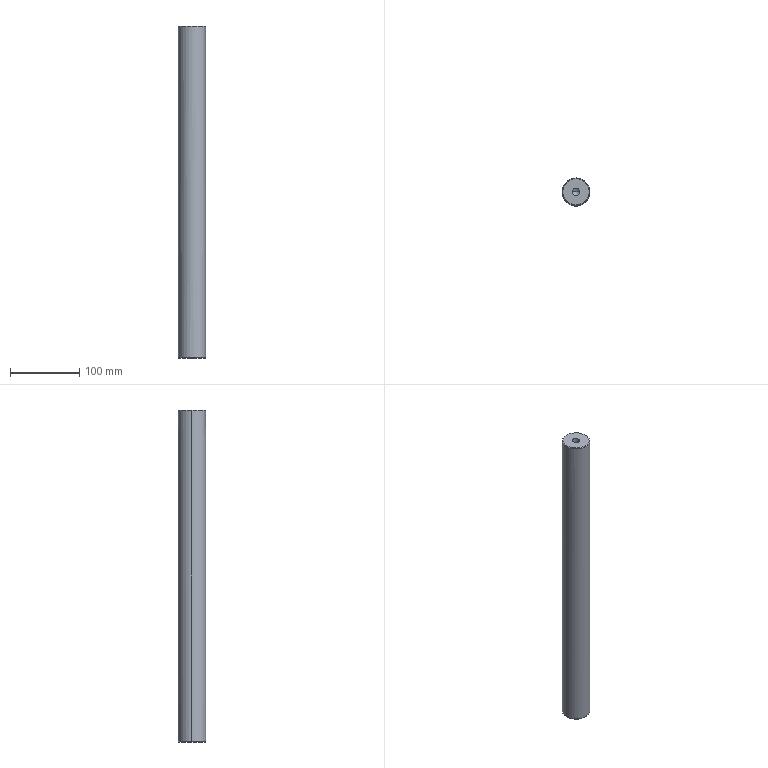Part | SolidWorks | features BaseBody 1 | 1 solid | 12 faces | box 40 x 40 x 480 mm | volume 600589 mm3 | cone 6 | cylinder 4 | plane 2 | commonest cylinder face diameters 10.2 x2 40 x2
STEP:
#1=CARTESIAN_POINT('',(0.,20.,479.));
#2=VERTEX_POINT('',#1);
#3=CARTESIAN_POINT('',(20.,0.,479.));
#4=VERTEX_POINT('',#3);
#5=CARTESIAN_POINT('',(0.,0.,479.));
#6=DIRECTION('',(0.,0.,-1.));
#7=DIRECTION('',(-1.,0.,0.));
#8=AXIS2_PLACEMENT_3D('',#5,#6,#7);
#9=CIRCLE('',#8,20.);
#10=EDGE_CURVE('',#2,#4,#9,.T.);
#11=ORIENTED_EDGE('',*,*,#10,.T.);
#12=CARTESIAN_POINT('',(20.,0.,1.));
#13=VERTEX_POINT('',#12);
#14=CARTESIAN_POINT('',(20.,0.,480.));
#15=DIRECTION('',(0.,0.,-1.));
#16=VECTOR('',#15,1000.);
#17=LINE('',#14,#16);
#18=EDGE_CURVE('',#4,#13,#17,.T.);
#19=ORIENTED_EDGE('',*,*,#18,.T.);
#20=CARTESIAN_POINT('',(-20.,0.,1.));
#21=VERTEX_POINT('',#20);
#22=CARTESIAN_POINT('',(0.,0.,1.));
#23=DIRECTION('',(0.,0.,1.));
#24=DIRECTION('',(-1.,0.,0.));
#25=AXIS2_PLACEMENT_3D('',#22,#23,#24);
#26=CIRCLE('',#25,20.);
#27=EDGE_CURVE('',#13,#21,#26,.T.);
#28=ORIENTED_EDGE('',*,*,#27,.T.);
#29=CARTESIAN_POINT('',(-20.,0.,479.));
#30=VERTEX_POINT('',#29);
#31=CARTESIAN_POINT('',(-20.,0.,480.));
#32=DIRECTION('',(0.,0.,-1.));
#33=VECTOR('',#32,1000.);
#34=LINE('',#31,#33);
#35=EDGE_CURVE('',#30,#21,#34,.T.);
#36=ORIENTED_EDGE('',*,*,#35,.F.);
#37=CARTESIAN_POINT('',(0.,0.,479.));
#38=DIRECTION('',(0.,0.,-1.));
#39=DIRECTION('',(-1.,0.,0.));
#40=AXIS2_PLACEMENT_3D('',#37,#38,#39);
#41=CIRCLE('',#40,20.);
#42=EDGE_CURVE('',#30,#2,#41,.T.);
#43=ORIENTED_EDGE('',*,*,#42,.T.);
#44=EDGE_LOOP('',(#11,#19,#28,#36,#43));
#45=FACE_OUTER_BOUND('',#44,.T.);
#46=CARTESIAN_POINT('',(0.,0.,480.));
#47=DIRECTION('',(0.,0.,-1.));
#48=DIRECTION('',(-1.,0.,0.));
#49=AXIS2_PLACEMENT_3D('',#46,#47,#48);
#50=CYLINDRICAL_SURFACE('',#49,20.);
#51=ADVANCED_FACE('',(#45),#50,.T.);
#52=CARTESIAN_POINT('',(19.,0.,0.));
#53=VERTEX_POINT('',#52);
#54=CARTESIAN_POINT('',(-19.,0.,0.));
#55=VERTEX_POINT('',#54);
#56=CARTESIAN_POINT('',(0.,0.,0.));
#57=DIRECTION('',(0.,0.,1.));
#58=DIRECTION('',(1.,0.,0.));
#59=AXIS2_PLACEMENT_3D('',#56,#57,#58);
#60=CIRCLE('',#59,19.);
#61=EDGE_CURVE('',#53,#55,#60,.T.);
#62=ORIENTED_EDGE('',*,*,#61,.T.);
#63=CARTESIAN_POINT('',(-20.,0.,1.));
#64=DIRECTION('',(-0.7071,0.,0.7071));
#65=VECTOR('',#64,1000.);
#66=LINE('',#63,#65);
#67=EDGE_CURVE('',#55,#21,#66,.T.);
#68=ORIENTED_EDGE('',*,*,#67,.T.);
#69=ORIENTED_EDGE('',*,*,#27,.F.);
#70=CARTESIAN_POINT('',(20.,0.,1.));
#71=DIRECTION('',(0.7071,0.,0.7071));
#72=VECTOR('',#71,1000.);
#73=LINE('',#70,#72);
#74=EDGE_CURVE('',#53,#13,#73,.T.);
#75=ORIENTED_EDGE('',*,*,#74,.F.);
#76=EDGE_LOOP('',(#62,#68,#69,#75));
#77=FACE_OUTER_BOUND('',#76,.T.);
#78=CARTESIAN_POINT('',(0.,0.,1.));
#79=DIRECTION('',(0.,0.,1.));
#80=DIRECTION('',(1.,0.,0.));
#81=AXIS2_PLACEMENT_3D('',#78,#79,#80);
#82=CONICAL_SURFACE('',#81,20.,0.7854);
#83=ADVANCED_FACE('',(#77),#82,.T.);
#84=CARTESIAN_POINT('',(0.,19.,480.));
#85=VERTEX_POINT('',#84);
#86=CARTESIAN_POINT('',(0.,-19.,480.));
#87=VERTEX_POINT('',#86);
#88=CARTESIAN_POINT('',(0.,0.,480.));
#89=DIRECTION('',(0.,0.,-1.));
#90=DIRECTION('',(0.,1.,0.));
#91=AXIS2_PLACEMENT_3D('',#88,#89,#90);
#92=CIRCLE('',#91,19.);
#93=EDGE_CURVE('',#85,#87,#92,.T.);
#94=ORIENTED_EDGE('',*,*,#93,.T.);
#95=CARTESIAN_POINT('',(0.,-20.,479.));
#96=VERTEX_POINT('',#95);
#97=CARTESIAN_POINT('',(0.,-20.,479.));
#98=DIRECTION('',(0.,-0.7071,-0.7071));
#99=VECTOR('',#98,1000.);
#100=LINE('',#97,#99);
#101=EDGE_CURVE('',#87,#96,#100,.T.);
#102=ORIENTED_EDGE('',*,*,#101,.T.);
#103=CARTESIAN_POINT('',(0.,0.,479.));
#104=DIRECTION('',(0.,0.,-1.));
#105=DIRECTION('',(-1.,0.,0.));
#106=AXIS2_PLACEMENT_3D('',#103,#104,#105);
#107=CIRCLE('',#106,20.);
#108=EDGE_CURVE('',#4,#96,#107,.T.);
#109=ORIENTED_EDGE('',*,*,#108,.F.);
#110=ORIENTED_EDGE('',*,*,#10,.F.);
#111=CARTESIAN_POINT('',(0.,20.,479.));
#112=DIRECTION('',(0.,0.7071,-0.7071));
#113=VECTOR('',#112,1000.);
#114=LINE('',#111,#113);
#115=EDGE_CURVE('',#85,#2,#114,.T.);
#116=ORIENTED_EDGE('',*,*,#115,.F.);
#117=EDGE_LOOP('',(#94,#102,#109,#110,#116));
#118=FACE_OUTER_BOUND('',#117,.T.);
#119=CARTESIAN_POINT('',(0.,0.,479.));
#120=DIRECTION('',(0.,0.,-1.));
#121=DIRECTION('',(0.,1.,0.));
#122=AXIS2_PLACEMENT_3D('',#119,#120,#121);
#123=CONICAL_SURFACE('',#122,20.,0.7854);
#124=ADVANCED_FACE('',(#118),#123,.T.);
#125=CARTESIAN_POINT('',(-5.1,0.,450.75));
#126=VERTEX_POINT('',#125);
#127=CARTESIAN_POINT('',(5.1,0.,450.75));
#128=VERTEX_POINT('',#127);
#129=CARTESIAN_POINT('',(0.,0.,450.75));
#130=DIRECTION('',(0.,0.,1.));
#131=DIRECTION('',(1.,0.,0.));
#132=AXIS2_PLACEMENT_3D('',#129,#130,#131);
#133=CIRCLE('',#132,5.1);
#134=EDGE_CURVE('',#126,#128,#133,.T.);
#135=ORIENTED_EDGE('',*,*,#134,.F.);
#136=CARTESIAN_POINT('',(-5.1,0.,480.));
#137=VERTEX_POINT('',#136);
#138=CARTESIAN_POINT('',(-5.1,0.,480.));
#139=DIRECTION('',(0.,0.,1.));
#140=VECTOR('',#139,1000.);
#141=LINE('',#138,#140);
#142=EDGE_CURVE('',#126,#137,#141,.T.);
#143=ORIENTED_EDGE('',*,*,#142,.T.);
#144=CARTESIAN_POINT('',(5.1,0.,480.));
#145=VERTEX_POINT('',#144);
#146=CARTESIAN_POINT('',(0.,0.,480.));
#147=DIRECTION('',(0.,0.,-1.));
#148=DIRECTION('',(1.,0.,0.));
#149=AXIS2_PLACEMENT_3D('',#146,#147,#148);
#150=CIRCLE('',#149,5.1);
#151=EDGE_CURVE('',#145,#137,#150,.T.);
#152=ORIENTED_EDGE('',*,*,#151,.F.);
#153=CARTESIAN_POINT('',(5.1,0.,480.));
#154=DIRECTION('',(0.,0.,1.));
#155=VECTOR('',#154,1000.);
#156=LINE('',#153,#155);
#157=EDGE_CURVE('',#128,#145,#156,.T.);
#158=ORIENTED_EDGE('',*,*,#157,.F.);
#159=EDGE_LOOP('',(#135,#143,#152,#158));
#160=FACE_OUTER_BOUND('',#159,.T.);
#161=CARTESIAN_POINT('',(0.,0.,480.));
#162=DIRECTION('',(0.,0.,1.));
#163=DIRECTION('',(1.,0.,0.));
#164=AXIS2_PLACEMENT_3D('',#161,#162,#163);
#165=CYLINDRICAL_SURFACE('',#164,5.1);
#166=ADVANCED_FACE('',(#160),#165,.F.);
#167=CARTESIAN_POINT('',(0.,0.,447.686));
#168=VERTEX_POINT('',#167);
#169=CARTESIAN_POINT('',(5.1,0.,450.75));
#170=DIRECTION('',(0.8572,0.,0.515));
#171=VECTOR('',#170,1000.);
#172=LINE('',#169,#171);
#173=EDGE_CURVE('',#168,#128,#172,.T.);
#174=ORIENTED_EDGE('',*,*,#173,.F.);
#175=CARTESIAN_POINT('',(-5.1,0.,450.75));
#176=DIRECTION('',(-0.8572,0.,0.515));
#177=VECTOR('',#176,1000.);
#178=LINE('',#175,#177);
#179=EDGE_CURVE('',#168,#126,#178,.T.);
#180=ORIENTED_EDGE('',*,*,#179,.T.);
#181=ORIENTED_EDGE('',*,*,#134,.T.);
#182=EDGE_LOOP('',(#174,#180,#181));
#183=FACE_OUTER_BOUND('',#182,.T.);
#184=CARTESIAN_POINT('',(0.,0.,450.75));
#185=DIRECTION('',(0.,0.,1.));
#186=DIRECTION('',(1.,0.,0.));
#187=AXIS2_PLACEMENT_3D('',#184,#185,#186);
#188=CONICAL_SURFACE('',#187,5.1,1.03);
#189=ADVANCED_FACE('',(#183),#188,.F.);
#190=ORIENTED_EDGE('',*,*,#18,.F.);
#191=ORIENTED_EDGE('',*,*,#108,.T.);
#192=CARTESIAN_POINT('',(0.,0.,479.));
#193=DIRECTION('',(0.,0.,-1.));
#194=DIRECTION('',(-1.,0.,0.));
#195=AXIS2_PLACEMENT_3D('',#192,#193,#194);
#196=CIRCLE('',#195,20.);
#197=EDGE_CURVE('',#96,#30,#196,.T.);
#198=ORIENTED_EDGE('',*,*,#197,.T.);
#199=ORIENTED_EDGE('',*,*,#35,.T.);
#200=CARTESIAN_POINT('',(0.,0.,1.));
#201=DIRECTION('',(0.,0.,1.));
#202=DIRECTION('',(-1.,0.,0.));
#203=AXIS2_PLACEMENT_3D('',#200,#201,#202);
#204=CIRCLE('',#203,20.);
#205=EDGE_CURVE('',#21,#13,#204,.T.);
#206=ORIENTED_EDGE('',*,*,#205,.T.);
#207=EDGE_LOOP('',(#190,#191,#198,#199,#206));
#208=FACE_OUTER_BOUND('',#207,.T.);
#209=CARTESIAN_POINT('',(0.,0.,480.));
#210=DIRECTION('',(0.,0.,-1.));
#211=DIRECTION('',(-1.,0.,0.));
#212=AXIS2_PLACEMENT_3D('',#209,#210,#211);
#213=CYLINDRICAL_SURFACE('',#212,20.);
#214=ADVANCED_FACE('',(#208),#213,.T.);
#215=ORIENTED_EDGE('',*,*,#67,.F.);
#216=CARTESIAN_POINT('',(0.,0.,0.));
#217=DIRECTION('',(0.,0.,1.));
#218=DIRECTION('',(1.,0.,0.));
#219=AXIS2_PLACEMENT_3D('',#216,#217,#218);
#220=CIRCLE('',#219,19.);
#221=EDGE_CURVE('',#55,#53,#220,.T.);
#222=ORIENTED_EDGE('',*,*,#221,.T.);
#223=ORIENTED_EDGE('',*,*,#74,.T.);
#224=ORIENTED_EDGE('',*,*,#205,.F.);
#225=EDGE_LOOP('',(#215,#222,#223,#224));
#226=FACE_OUTER_BOUND('',#225,.T.);
#227=CARTESIAN_POINT('',(0.,0.,1.));
#228=DIRECTION('',(0.,0.,1.));
#229=DIRECTION('',(1.,0.,0.));
#230=AXIS2_PLACEMENT_3D('',#227,#228,#229);
#231=CONICAL_SURFACE('',#230,20.,0.7854);
#232=ADVANCED_FACE('',(#226),#231,.T.);
#233=ORIENTED_EDGE('',*,*,#101,.F.);
#234=CARTESIAN_POINT('',(0.,0.,480.));
#235=DIRECTION('',(0.,0.,-1.));
#236=DIRECTION('',(0.,1.,0.));
#237=AXIS2_PLACEMENT_3D('',#234,#235,#236);
#238=CIRCLE('',#237,19.);
#239=EDGE_CURVE('',#87,#85,#238,.T.);
#240=ORIENTED_EDGE('',*,*,#239,.T.);
#241=ORIENTED_EDGE('',*,*,#115,.T.);
#242=ORIENTED_EDGE('',*,*,#42,.F.);
#243=ORIENTED_EDGE('',*,*,#197,.F.);
#244=EDGE_LOOP('',(#233,#240,#241,#242,#243));
#245=FACE_OUTER_BOUND('',#244,.T.);
#246=CARTESIAN_POINT('',(0.,0.,479.));
#247=DIRECTION('',(0.,0.,-1.));
#248=DIRECTION('',(0.,1.,0.));
#249=AXIS2_PLACEMENT_3D('',#246,#247,#248);
#250=CONICAL_SURFACE('',#249,20.,0.7854);
#251=ADVANCED_FACE('',(#245),#250,.T.);
#252=ORIENTED_EDGE('',*,*,#61,.F.);
#253=ORIENTED_EDGE('',*,*,#221,.F.);
#254=EDGE_LOOP('',(#252,#253));
#255=FACE_OUTER_BOUND('',#254,.T.);
#256=CARTESIAN_POINT('',(0.,0.,0.));
#257=DIRECTION('',(0.,0.,1.));
#258=DIRECTION('',(1.,0.,0.));
#259=AXIS2_PLACEMENT_3D('',#256,#257,#258);
#260=PLANE('',#259);
#261=ADVANCED_FACE('',(#255),#260,.F.);
#262=ORIENTED_EDGE('',*,*,#151,.T.);
#263=CARTESIAN_POINT('',(0.,0.,480.));
#264=DIRECTION('',(0.,0.,-1.));
#265=DIRECTION('',(1.,0.,0.));
#266=AXIS2_PLACEMENT_3D('',#263,#264,#265);
#267=CIRCLE('',#266,5.1);
#268=EDGE_CURVE('',#137,#145,#267,.T.);
#269=ORIENTED_EDGE('',*,*,#268,.T.);
#270=EDGE_LOOP('',(#262,#269));
#271=FACE_BOUND('',#270,.T.);
#272=ORIENTED_EDGE('',*,*,#93,.F.);
#273=ORIENTED_EDGE('',*,*,#239,.F.);
#274=EDGE_LOOP('',(#272,#273));
#275=FACE_OUTER_BOUND('',#274,.T.);
#276=CARTESIAN_POINT('',(0.,0.,480.));
#277=DIRECTION('',(0.,0.,1.));
#278=DIRECTION('',(1.,0.,0.));
#279=AXIS2_PLACEMENT_3D('',#276,#277,#278);
#280=PLANE('',#279);
#281=ADVANCED_FACE('',(#271,#275),#280,.T.);
#282=ORIENTED_EDGE('',*,*,#142,.F.);
#283=CARTESIAN_POINT('',(0.,0.,450.75));
#284=DIRECTION('',(0.,0.,1.));
#285=DIRECTION('',(1.,0.,0.));
#286=AXIS2_PLACEMENT_3D('',#283,#284,#285);
#287=CIRCLE('',#286,5.1);
#288=EDGE_CURVE('',#128,#126,#287,.T.);
#289=ORIENTED_EDGE('',*,*,#288,.F.);
#290=ORIENTED_EDGE('',*,*,#157,.T.);
#291=ORIENTED_EDGE('',*,*,#268,.F.);
#292=EDGE_LOOP('',(#282,#289,#290,#291));
#293=FACE_OUTER_BOUND('',#292,.T.);
#294=CARTESIAN_POINT('',(0.,0.,480.));
#295=DIRECTION('',(0.,0.,1.));
#296=DIRECTION('',(1.,0.,0.));
#297=AXIS2_PLACEMENT_3D('',#294,#295,#296);
#298=CYLINDRICAL_SURFACE('',#297,5.1);
#299=ADVANCED_FACE('',(#293),#298,.F.);
#300=ORIENTED_EDGE('',*,*,#179,.F.);
#301=ORIENTED_EDGE('',*,*,#173,.T.);
#302=ORIENTED_EDGE('',*,*,#288,.T.);
#303=EDGE_LOOP('',(#300,#301,#302));
#304=FACE_OUTER_BOUND('',#303,.T.);
#305=CARTESIAN_POINT('',(0.,0.,450.75));
#306=DIRECTION('',(0.,0.,1.));
#307=DIRECTION('',(1.,0.,0.));
#308=AXIS2_PLACEMENT_3D('',#305,#306,#307);
#309=CONICAL_SURFACE('',#308,5.1,1.03);
#310=ADVANCED_FACE('',(#304),#309,.F.);
#311=CLOSED_SHELL('',(#51,#83,#124,#166,#189,#214,#232,#251,#261,#281,#299,#310));
#312=MANIFOLD_SOLID_BREP('',#311);
#313=CARTESIAN_POINT('',(0.,0.,0.));
#314=DIRECTION('',(0.,0.,1.));
#315=DIRECTION('',(1.,0.,0.));
#316=AXIS2_PLACEMENT_3D('',#313,#314,#315);
#317=(LENGTH_UNIT()NAMED_UNIT(*)SI_UNIT(.MILLI.,.METRE.));
#318=UNCERTAINTY_MEASURE_WITH_UNIT(LENGTH_MEASURE(0.00001),#317,'','');
#319=(NAMED_UNIT(*)PLANE_ANGLE_UNIT()SI_UNIT($,.RADIAN.));
#320=(NAMED_UNIT(*)SI_UNIT($,.STERADIAN.)SOLID_ANGLE_UNIT());
#321=(GEOMETRIC_REPRESENTATION_CONTEXT(3)GLOBAL_UNCERTAINTY_ASSIGNED_CONTEXT((#318))GLOBAL_UNIT_ASSIGNED_CONTEXT((#317,#319,#320))REPRESENTATION_CONTEXT('',''));
#322=ADVANCED_BREP_SHAPE_REPRESENTATION('',(#312,#316),#321);